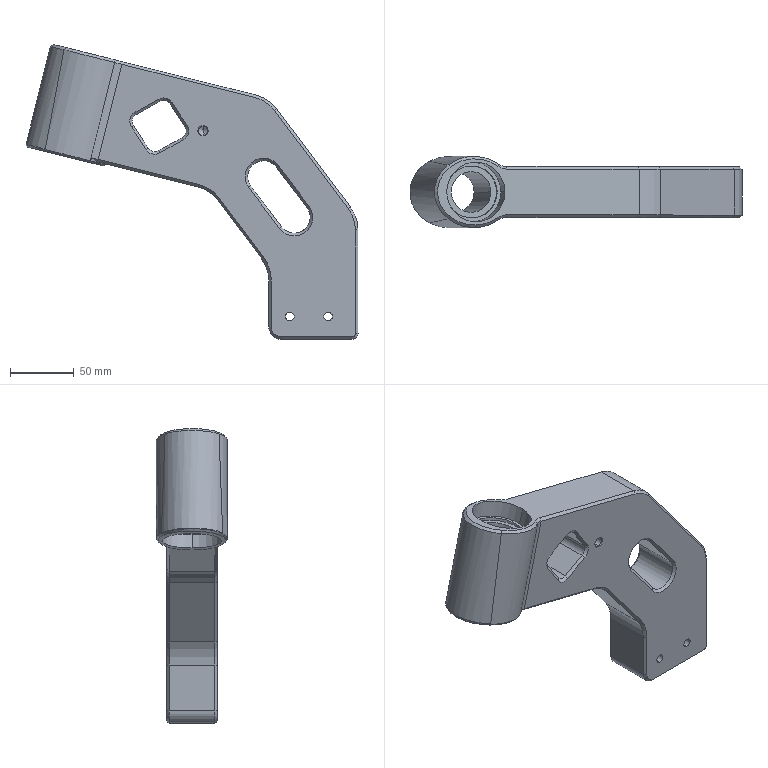Part | SolidWorks | features BaseBody 1 | 1 solid | 148 faces | box 260.675 x 55.997 x 231.421 mm | volume 878681 mm3 | cone 50 | plane 48 | cylinder 44 | spline 6 | commonest cylinder face diameters 6.8 x14 12 x5 41 x4 47 x4 20 x3 25 x3